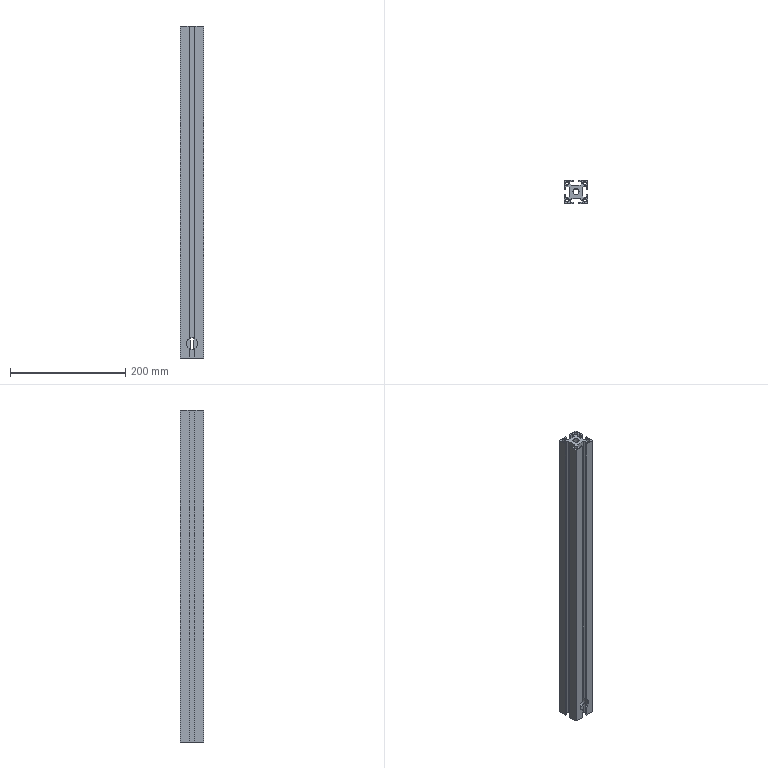Part | SolidWorks | features BaseBody 1 | 1 solid | 78 faces | box 40 x 40 x 575 mm | volume 445700 mm3 | plane 62 | cylinder 16 | commonest cylinder face diameters 6 x8 20.5 x6 10.5 x2